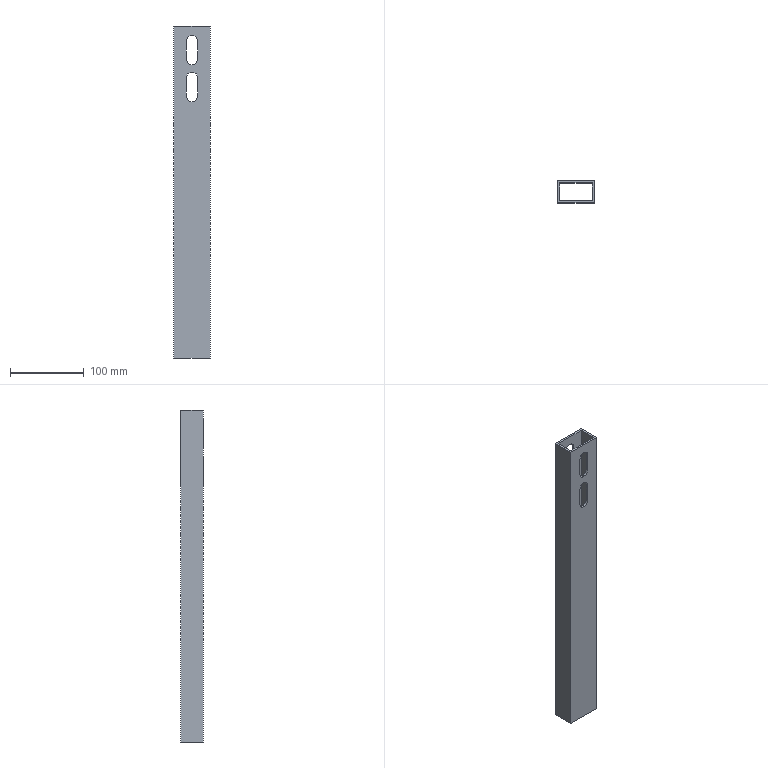Part | SolidWorks | features ICE 2, Extrusion 1 | 1 solid | 30 faces | box 50 x 30 x 450 mm | volume 193179 mm3 | plane 18 | cylinder 12 | commonest cylinder face diameters 15 x12
STEP:
#1=CARTESIAN_POINT('',(32.5,3.,355.));
#2=VERTEX_POINT('',#1);
#3=CARTESIAN_POINT('',(25.,3.,347.5));
#4=VERTEX_POINT('',#3);
#5=CARTESIAN_POINT('',(25.,3.,355.));
#6=DIRECTION('',(0.,1.,0.));
#7=DIRECTION('',(0.,0.,1.));
#8=AXIS2_PLACEMENT_3D('',#5,#6,#7);
#9=CIRCLE('',#8,7.5);
#10=EDGE_CURVE('',#2,#4,#9,.T.);
#11=ORIENTED_EDGE('',*,*,#10,.T.);
#12=CARTESIAN_POINT('',(25.,0.,347.5));
#13=VERTEX_POINT('',#12);
#14=CARTESIAN_POINT('',(25.,450.,347.5));
#15=DIRECTION('',(0.,-1.,0.));
#16=VECTOR('',#15,1000.);
#17=LINE('',#14,#16);
#18=EDGE_CURVE('',#4,#13,#17,.T.);
#19=ORIENTED_EDGE('',*,*,#18,.T.);
#20=CARTESIAN_POINT('',(32.5,0.,355.));
#21=VERTEX_POINT('',#20);
#22=CARTESIAN_POINT('',(25.,0.,355.));
#23=DIRECTION('',(0.,-1.,0.));
#24=DIRECTION('',(0.,0.,-1.));
#25=AXIS2_PLACEMENT_3D('',#22,#23,#24);
#26=CIRCLE('',#25,7.5);
#27=EDGE_CURVE('',#13,#21,#26,.T.);
#28=ORIENTED_EDGE('',*,*,#27,.T.);
#29=CARTESIAN_POINT('',(32.5,450.,355.));
#30=DIRECTION('',(0.,-1.,0.));
#31=VECTOR('',#30,1000.);
#32=LINE('',#29,#31);
#33=EDGE_CURVE('',#2,#21,#32,.T.);
#34=ORIENTED_EDGE('',*,*,#33,.F.);
#35=EDGE_LOOP('',(#11,#19,#28,#34));
#36=FACE_OUTER_BOUND('',#35,.T.);
#37=CARTESIAN_POINT('',(25.,450.,355.));
#38=DIRECTION('',(0.,-1.,0.));
#39=DIRECTION('',(0.,0.,-1.));
#40=AXIS2_PLACEMENT_3D('',#37,#38,#39);
#41=CYLINDRICAL_SURFACE('',#40,7.5);
#42=ADVANCED_FACE('',(#36),#41,.F.);
#43=CARTESIAN_POINT('',(25.,30.,347.5));
#44=VERTEX_POINT('',#43);
#45=CARTESIAN_POINT('',(32.5,30.,355.));
#46=VERTEX_POINT('',#45);
#47=CARTESIAN_POINT('',(25.,30.,355.));
#48=DIRECTION('',(0.,-1.,0.));
#49=DIRECTION('',(0.,0.,-1.));
#50=AXIS2_PLACEMENT_3D('',#47,#48,#49);
#51=CIRCLE('',#50,7.5);
#52=EDGE_CURVE('',#44,#46,#51,.T.);
#53=ORIENTED_EDGE('',*,*,#52,.F.);
#54=CARTESIAN_POINT('',(25.,27.,347.5));
#55=VERTEX_POINT('',#54);
#56=CARTESIAN_POINT('',(25.,450.,347.5));
#57=DIRECTION('',(0.,-1.,0.));
#58=VECTOR('',#57,1000.);
#59=LINE('',#56,#58);
#60=EDGE_CURVE('',#44,#55,#59,.T.);
#61=ORIENTED_EDGE('',*,*,#60,.T.);
#62=CARTESIAN_POINT('',(32.5,27.,355.));
#63=VERTEX_POINT('',#62);
#64=CARTESIAN_POINT('',(25.,27.,355.));
#65=DIRECTION('',(0.,-1.,0.));
#66=DIRECTION('',(0.,0.,-1.));
#67=AXIS2_PLACEMENT_3D('',#64,#65,#66);
#68=CIRCLE('',#67,7.5);
#69=EDGE_CURVE('',#55,#63,#68,.T.);
#70=ORIENTED_EDGE('',*,*,#69,.T.);
#71=CARTESIAN_POINT('',(32.5,450.,355.));
#72=DIRECTION('',(0.,-1.,0.));
#73=VECTOR('',#72,1000.);
#74=LINE('',#71,#73);
#75=EDGE_CURVE('',#46,#63,#74,.T.);
#76=ORIENTED_EDGE('',*,*,#75,.F.);
#77=EDGE_LOOP('',(#53,#61,#70,#76));
#78=FACE_OUTER_BOUND('',#77,.T.);
#79=CARTESIAN_POINT('',(25.,450.,355.));
#80=DIRECTION('',(0.,-1.,0.));
#81=DIRECTION('',(0.,0.,-1.));
#82=AXIS2_PLACEMENT_3D('',#79,#80,#81);
#83=CYLINDRICAL_SURFACE('',#82,7.5);
#84=ADVANCED_FACE('',(#78),#83,.F.);
#85=CARTESIAN_POINT('',(32.5,3.,405.));
#86=VERTEX_POINT('',#85);
#87=CARTESIAN_POINT('',(25.,3.,397.5));
#88=VERTEX_POINT('',#87);
#89=CARTESIAN_POINT('',(25.,3.,405.));
#90=DIRECTION('',(0.,1.,0.));
#91=DIRECTION('',(0.,0.,1.));
#92=AXIS2_PLACEMENT_3D('',#89,#90,#91);
#93=CIRCLE('',#92,7.5);
#94=EDGE_CURVE('',#86,#88,#93,.T.);
#95=ORIENTED_EDGE('',*,*,#94,.T.);
#96=CARTESIAN_POINT('',(25.,0.,397.5));
#97=VERTEX_POINT('',#96);
#98=CARTESIAN_POINT('',(25.,450.,397.5));
#99=DIRECTION('',(0.,-1.,0.));
#100=VECTOR('',#99,1000.);
#101=LINE('',#98,#100);
#102=EDGE_CURVE('',#88,#97,#101,.T.);
#103=ORIENTED_EDGE('',*,*,#102,.T.);
#104=CARTESIAN_POINT('',(32.5,0.,405.));
#105=VERTEX_POINT('',#104);
#106=CARTESIAN_POINT('',(25.,0.,405.));
#107=DIRECTION('',(0.,-1.,0.));
#108=DIRECTION('',(0.,0.,-1.));
#109=AXIS2_PLACEMENT_3D('',#106,#107,#108);
#110=CIRCLE('',#109,7.5);
#111=EDGE_CURVE('',#97,#105,#110,.T.);
#112=ORIENTED_EDGE('',*,*,#111,.T.);
#113=CARTESIAN_POINT('',(32.5,450.,405.));
#114=DIRECTION('',(0.,-1.,0.));
#115=VECTOR('',#114,1000.);
#116=LINE('',#113,#115);
#117=EDGE_CURVE('',#86,#105,#116,.T.);
#118=ORIENTED_EDGE('',*,*,#117,.F.);
#119=EDGE_LOOP('',(#95,#103,#112,#118));
#120=FACE_OUTER_BOUND('',#119,.T.);
#121=CARTESIAN_POINT('',(25.,450.,405.));
#122=DIRECTION('',(0.,-1.,0.));
#123=DIRECTION('',(0.,0.,-1.));
#124=AXIS2_PLACEMENT_3D('',#121,#122,#123);
#125=CYLINDRICAL_SURFACE('',#124,7.5);
#126=ADVANCED_FACE('',(#120),#125,.F.);
#127=CARTESIAN_POINT('',(25.,30.,397.5));
#128=VERTEX_POINT('',#127);
#129=CARTESIAN_POINT('',(32.5,30.,405.));
#130=VERTEX_POINT('',#129);
#131=CARTESIAN_POINT('',(25.,30.,405.));
#132=DIRECTION('',(0.,-1.,0.));
#133=DIRECTION('',(0.,0.,-1.));
#134=AXIS2_PLACEMENT_3D('',#131,#132,#133);
#135=CIRCLE('',#134,7.5);
#136=EDGE_CURVE('',#128,#130,#135,.T.);
#137=ORIENTED_EDGE('',*,*,#136,.F.);
#138=CARTESIAN_POINT('',(25.,27.,397.5));
#139=VERTEX_POINT('',#138);
#140=CARTESIAN_POINT('',(25.,450.,397.5));
#141=DIRECTION('',(0.,-1.,0.));
#142=VECTOR('',#141,1000.);
#143=LINE('',#140,#142);
#144=EDGE_CURVE('',#128,#139,#143,.T.);
#145=ORIENTED_EDGE('',*,*,#144,.T.);
#146=CARTESIAN_POINT('',(32.5,27.,405.));
#147=VERTEX_POINT('',#146);
#148=CARTESIAN_POINT('',(25.,27.,405.));
#149=DIRECTION('',(0.,-1.,0.));
#150=DIRECTION('',(0.,0.,-1.));
#151=AXIS2_PLACEMENT_3D('',#148,#149,#150);
#152=CIRCLE('',#151,7.5);
#153=EDGE_CURVE('',#139,#147,#152,.T.);
#154=ORIENTED_EDGE('',*,*,#153,.T.);
#155=CARTESIAN_POINT('',(32.5,450.,405.));
#156=DIRECTION('',(0.,-1.,0.));
#157=VECTOR('',#156,1000.);
#158=LINE('',#155,#157);
#159=EDGE_CURVE('',#130,#147,#158,.T.);
#160=ORIENTED_EDGE('',*,*,#159,.F.);
#161=EDGE_LOOP('',(#137,#145,#154,#160));
#162=FACE_OUTER_BOUND('',#161,.T.);
#163=CARTESIAN_POINT('',(25.,450.,405.));
#164=DIRECTION('',(0.,-1.,0.));
#165=DIRECTION('',(0.,0.,-1.));
#166=AXIS2_PLACEMENT_3D('',#163,#164,#165);
#167=CYLINDRICAL_SURFACE('',#166,7.5);
#168=ADVANCED_FACE('',(#162),#167,.F.);
#169=CARTESIAN_POINT('',(0.,30.,450.));
#170=VERTEX_POINT('',#169);
#171=CARTESIAN_POINT('',(0.,0.,450.));
#172=VERTEX_POINT('',#171);
#173=CARTESIAN_POINT('',(0.,30.,450.));
#174=DIRECTION('',(0.,-1.,0.));
#175=VECTOR('',#174,1000.);
#176=LINE('',#173,#175);
#177=EDGE_CURVE('',#170,#172,#176,.T.);
#178=ORIENTED_EDGE('',*,*,#177,.T.);
#179=CARTESIAN_POINT('',(50.,0.,450.));
#180=VERTEX_POINT('',#179);
#181=CARTESIAN_POINT('',(0.,0.,450.));
#182=DIRECTION('',(1.,0.,0.));
#183=VECTOR('',#182,1000.);
#184=LINE('',#181,#183);
#185=EDGE_CURVE('',#172,#180,#184,.T.);
#186=ORIENTED_EDGE('',*,*,#185,.T.);
#187=CARTESIAN_POINT('',(50.,30.,450.));
#188=VERTEX_POINT('',#187);
#189=CARTESIAN_POINT('',(50.,0.,450.));
#190=DIRECTION('',(0.,1.,0.));
#191=VECTOR('',#190,1000.);
#192=LINE('',#189,#191);
#193=EDGE_CURVE('',#180,#188,#192,.T.);
#194=ORIENTED_EDGE('',*,*,#193,.T.);
#195=CARTESIAN_POINT('',(50.,30.,450.));
#196=DIRECTION('',(-1.,0.,0.));
#197=VECTOR('',#196,1000.);
#198=LINE('',#195,#197);
#199=EDGE_CURVE('',#188,#170,#198,.T.);
#200=ORIENTED_EDGE('',*,*,#199,.T.);
#201=EDGE_LOOP('',(#178,#186,#194,#200));
#202=FACE_OUTER_BOUND('',#201,.T.);
#203=CARTESIAN_POINT('',(3.,3.,450.));
#204=VERTEX_POINT('',#203);
#205=CARTESIAN_POINT('',(47.,3.,450.));
#206=VERTEX_POINT('',#205);
#207=CARTESIAN_POINT('',(3.,3.,450.));
#208=DIRECTION('',(1.,0.,0.));
#209=VECTOR('',#208,1000.);
#210=LINE('',#207,#209);
#211=EDGE_CURVE('',#204,#206,#210,.T.);
#212=ORIENTED_EDGE('',*,*,#211,.F.);
#213=CARTESIAN_POINT('',(3.,27.,450.));
#214=VERTEX_POINT('',#213);
#215=CARTESIAN_POINT('',(3.,27.,450.));
#216=DIRECTION('',(0.,-1.,0.));
#217=VECTOR('',#216,1000.);
#218=LINE('',#215,#217);
#219=EDGE_CURVE('',#214,#204,#218,.T.);
#220=ORIENTED_EDGE('',*,*,#219,.F.);
#221=CARTESIAN_POINT('',(47.,27.,450.));
#222=VERTEX_POINT('',#221);
#223=CARTESIAN_POINT('',(47.,27.,450.));
#224=DIRECTION('',(-1.,0.,0.));
#225=VECTOR('',#224,1000.);
#226=LINE('',#223,#225);
#227=EDGE_CURVE('',#222,#214,#226,.T.);
#228=ORIENTED_EDGE('',*,*,#227,.F.);
#229=CARTESIAN_POINT('',(47.,3.,450.));
#230=DIRECTION('',(0.,1.,0.));
#231=VECTOR('',#230,1000.);
#232=LINE('',#229,#231);
#233=EDGE_CURVE('',#206,#222,#232,.T.);
#234=ORIENTED_EDGE('',*,*,#233,.F.);
#235=EDGE_LOOP('',(#212,#220,#228,#234));
#236=FACE_BOUND('',#235,.T.);
#237=CARTESIAN_POINT('',(0.,0.,450.));
#238=DIRECTION('',(0.,0.,1.));
#239=DIRECTION('',(1.,0.,0.));
#240=AXIS2_PLACEMENT_3D('',#237,#238,#239);
#241=PLANE('',#240);
#242=ADVANCED_FACE('',(#202,#236),#241,.T.);
#243=CARTESIAN_POINT('',(0.,30.,0.));
#244=VERTEX_POINT('',#243);
#245=CARTESIAN_POINT('',(0.,0.,0.));
#246=VERTEX_POINT('',#245);
#247=CARTESIAN_POINT('',(0.,30.,0.));
#248=DIRECTION('',(0.,-1.,0.));
#249=VECTOR('',#248,1000.);
#250=LINE('',#247,#249);
#251=EDGE_CURVE('',#244,#246,#250,.T.);
#252=ORIENTED_EDGE('',*,*,#251,.F.);
#253=CARTESIAN_POINT('',(50.,30.,0.));
#254=VERTEX_POINT('',#253);
#255=CARTESIAN_POINT('',(50.,30.,0.));
#256=DIRECTION('',(-1.,0.,0.));
#257=VECTOR('',#256,1000.);
#258=LINE('',#255,#257);
#259=EDGE_CURVE('',#254,#244,#258,.T.);
#260=ORIENTED_EDGE('',*,*,#259,.F.);
#261=CARTESIAN_POINT('',(50.,0.,0.));
#262=VERTEX_POINT('',#261);
#263=CARTESIAN_POINT('',(50.,0.,0.));
#264=DIRECTION('',(0.,1.,0.));
#265=VECTOR('',#264,1000.);
#266=LINE('',#263,#265);
#267=EDGE_CURVE('',#262,#254,#266,.T.);
#268=ORIENTED_EDGE('',*,*,#267,.F.);
#269=CARTESIAN_POINT('',(0.,0.,0.));
#270=DIRECTION('',(1.,0.,0.));
#271=VECTOR('',#270,1000.);
#272=LINE('',#269,#271);
#273=EDGE_CURVE('',#246,#262,#272,.T.);
#274=ORIENTED_EDGE('',*,*,#273,.F.);
#275=EDGE_LOOP('',(#252,#260,#268,#274));
#276=FACE_OUTER_BOUND('',#275,.T.);
#277=CARTESIAN_POINT('',(3.,27.,0.));
#278=VERTEX_POINT('',#277);
#279=CARTESIAN_POINT('',(3.,3.,0.));
#280=VERTEX_POINT('',#279);
#281=CARTESIAN_POINT('',(3.,27.,0.));
#282=DIRECTION('',(0.,-1.,0.));
#283=VECTOR('',#282,1000.);
#284=LINE('',#281,#283);
#285=EDGE_CURVE('',#278,#280,#284,.T.);
#286=ORIENTED_EDGE('',*,*,#285,.T.);
#287=CARTESIAN_POINT('',(47.,3.,0.));
#288=VERTEX_POINT('',#287);
#289=CARTESIAN_POINT('',(3.,3.,0.));
#290=DIRECTION('',(1.,0.,0.));
#291=VECTOR('',#290,1000.);
#292=LINE('',#289,#291);
#293=EDGE_CURVE('',#280,#288,#292,.T.);
#294=ORIENTED_EDGE('',*,*,#293,.T.);
#295=CARTESIAN_POINT('',(47.,27.,0.));
#296=VERTEX_POINT('',#295);
#297=CARTESIAN_POINT('',(47.,3.,0.));
#298=DIRECTION('',(0.,1.,0.));
#299=VECTOR('',#298,1000.);
#300=LINE('',#297,#299);
#301=EDGE_CURVE('',#288,#296,#300,.T.);
#302=ORIENTED_EDGE('',*,*,#301,.T.);
#303=CARTESIAN_POINT('',(47.,27.,0.));
#304=DIRECTION('',(-1.,0.,0.));
#305=VECTOR('',#304,1000.);
#306=LINE('',#303,#305);
#307=EDGE_CURVE('',#296,#278,#306,.T.);
#308=ORIENTED_EDGE('',*,*,#307,.T.);
#309=EDGE_LOOP('',(#286,#294,#302,#308));
#310=FACE_BOUND('',#309,.T.);
#311=CARTESIAN_POINT('',(0.,0.,0.));
#312=DIRECTION('',(0.,0.,1.));
#313=DIRECTION('',(1.,0.,0.));
#314=AXIS2_PLACEMENT_3D('',#311,#312,#313);
#315=PLANE('',#314);
#316=ADVANCED_FACE('',(#276,#310),#315,.F.);
#317=ORIENTED_EDGE('',*,*,#251,.T.);
#318=CARTESIAN_POINT('',(0.,0.,450.));
#319=DIRECTION('',(0.,0.,-1.));
#320=VECTOR('',#319,1000.);
#321=LINE('',#318,#320);
#322=EDGE_CURVE('',#172,#246,#321,.T.);
#323=ORIENTED_EDGE('',*,*,#322,.F.);
#324=ORIENTED_EDGE('',*,*,#177,.F.);
#325=CARTESIAN_POINT('',(0.,30.,450.));
#326=DIRECTION('',(0.,0.,-1.));
#327=VECTOR('',#326,1000.);
#328=LINE('',#325,#327);
#329=EDGE_CURVE('',#170,#244,#328,.T.);
#330=ORIENTED_EDGE('',*,*,#329,.T.);
#331=EDGE_LOOP('',(#317,#323,#324,#330));
#332=FACE_OUTER_BOUND('',#331,.T.);
#333=CARTESIAN_POINT('',(0.,30.,450.));
#334=DIRECTION('',(1.,0.,0.));
#335=DIRECTION('',(0.,0.,-1.));
#336=AXIS2_PLACEMENT_3D('',#333,#334,#335);
#337=PLANE('',#336);
#338=ADVANCED_FACE('',(#332),#337,.F.);
#339=CARTESIAN_POINT('',(32.5,0.,380.));
#340=VERTEX_POINT('',#339);
#341=CARTESIAN_POINT('',(32.5,0.,380.));
#342=DIRECTION('',(0.,0.,1.));
#343=VECTOR('',#342,1000.);
#344=LINE('',#341,#343);
#345=EDGE_CURVE('',#21,#340,#344,.T.);
#346=ORIENTED_EDGE('',*,*,#345,.F.);
#347=ORIENTED_EDGE('',*,*,#27,.F.);
#348=CARTESIAN_POINT('',(17.5,0.,355.));
#349=VERTEX_POINT('',#348);
#350=CARTESIAN_POINT('',(25.,0.,355.));
#351=DIRECTION('',(0.,-1.,0.));
#352=DIRECTION('',(0.,0.,-1.));
#353=AXIS2_PLACEMENT_3D('',#350,#351,#352);
#354=CIRCLE('',#353,7.5);
#355=EDGE_CURVE('',#349,#13,#354,.T.);
#356=ORIENTED_EDGE('',*,*,#355,.F.);
#357=CARTESIAN_POINT('',(17.5,0.,380.));
#358=VERTEX_POINT('',#357);
#359=CARTESIAN_POINT('',(17.5,0.,380.));
#360=DIRECTION('',(0.,0.,-1.));
#361=VECTOR('',#360,1000.);
#362=LINE('',#359,#361);
#363=EDGE_CURVE('',#358,#349,#362,.T.);
#364=ORIENTED_EDGE('',*,*,#363,.F.);
#365=CARTESIAN_POINT('',(25.,0.,380.));
#366=DIRECTION('',(0.,-1.,0.));
#367=DIRECTION('',(0.,0.,-1.));
#368=AXIS2_PLACEMENT_3D('',#365,#366,#367);
#369=CIRCLE('',#368,7.5);
#370=EDGE_CURVE('',#340,#358,#369,.T.);
#371=ORIENTED_EDGE('',*,*,#370,.F.);
#372=EDGE_LOOP('',(#346,#347,#356,#364,#371));
#373=FACE_BOUND('',#372,.T.);
#374=CARTESIAN_POINT('',(17.5,0.,430.));
#375=VERTEX_POINT('',#374);
#376=CARTESIAN_POINT('',(17.5,0.,405.));
#377=VERTEX_POINT('',#376);
#378=CARTESIAN_POINT('',(17.5,0.,430.));
#379=DIRECTION('',(0.,0.,-1.));
#380=VECTOR('',#379,1000.);
#381=LINE('',#378,#380);
#382=EDGE_CURVE('',#375,#377,#381,.T.);
#383=ORIENTED_EDGE('',*,*,#382,.F.);
#384=CARTESIAN_POINT('',(32.5,0.,430.));
#385=VERTEX_POINT('',#384);
#386=CARTESIAN_POINT('',(25.,0.,430.));
#387=DIRECTION('',(0.,-1.,0.));
#388=DIRECTION('',(0.,0.,-1.));
#389=AXIS2_PLACEMENT_3D('',#386,#387,#388);
#390=CIRCLE('',#389,7.5);
#391=EDGE_CURVE('',#385,#375,#390,.T.);
#392=ORIENTED_EDGE('',*,*,#391,.F.);
#393=CARTESIAN_POINT('',(32.5,0.,430.));
#394=DIRECTION('',(0.,0.,1.));
#395=VECTOR('',#394,1000.);
#396=LINE('',#393,#395);
#397=EDGE_CURVE('',#105,#385,#396,.T.);
#398=ORIENTED_EDGE('',*,*,#397,.F.);
#399=ORIENTED_EDGE('',*,*,#111,.F.);
#400=CARTESIAN_POINT('',(25.,0.,405.));
#401=DIRECTION('',(0.,-1.,0.));
#402=DIRECTION('',(0.,0.,-1.));
#403=AXIS2_PLACEMENT_3D('',#400,#401,#402);
#404=CIRCLE('',#403,7.5);
#405=EDGE_CURVE('',#377,#97,#404,.T.);
#406=ORIENTED_EDGE('',*,*,#405,.F.);
#407=EDGE_LOOP('',(#383,#392,#398,#399,#406));
#408=FACE_BOUND('',#407,.T.);
#409=ORIENTED_EDGE('',*,*,#273,.T.);
#410=CARTESIAN_POINT('',(50.,0.,450.));
#411=DIRECTION('',(0.,0.,-1.));
#412=VECTOR('',#411,1000.);
#413=LINE('',#410,#412);
#414=EDGE_CURVE('',#180,#262,#413,.T.);
#415=ORIENTED_EDGE('',*,*,#414,.F.);
#416=ORIENTED_EDGE('',*,*,#185,.F.);
#417=ORIENTED_EDGE('',*,*,#322,.T.);
#418=EDGE_LOOP('',(#409,#415,#416,#417));
#419=FACE_OUTER_BOUND('',#418,.T.);
#420=CARTESIAN_POINT('',(0.,0.,450.));
#421=DIRECTION('',(0.,1.,0.));
#422=DIRECTION('',(0.,0.,1.));
#423=AXIS2_PLACEMENT_3D('',#420,#421,#422);
#424=PLANE('',#423);
#425=ADVANCED_FACE('',(#373,#408,#419),#424,.F.);
#426=ORIENTED_EDGE('',*,*,#267,.T.);
#427=CARTESIAN_POINT('',(50.,30.,450.));
#428=DIRECTION('',(0.,0.,-1.));
#429=VECTOR('',#428,1000.);
#430=LINE('',#427,#429);
#431=EDGE_CURVE('',#188,#254,#430,.T.);
#432=ORIENTED_EDGE('',*,*,#431,.F.);
#433=ORIENTED_EDGE('',*,*,#193,.F.);
#434=ORIENTED_EDGE('',*,*,#414,.T.);
#435=EDGE_LOOP('',(#426,#432,#433,#434));
#436=FACE_OUTER_BOUND('',#435,.T.);
#437=CARTESIAN_POINT('',(50.,0.,450.));
#438=DIRECTION('',(-1.,0.,0.));
#439=DIRECTION('',(0.,0.,1.));
#440=AXIS2_PLACEMENT_3D('',#437,#438,#439);
#441=PLANE('',#440);
#442=ADVANCED_FACE('',(#436),#441,.F.);
#443=CARTESIAN_POINT('',(17.5,30.,380.));
#444=VERTEX_POINT('',#443);
#445=CARTESIAN_POINT('',(17.5,30.,355.));
#446=VERTEX_POINT('',#445);
#447=CARTESIAN_POINT('',(17.5,30.,450.));
#448=DIRECTION('',(0.,0.,-1.));
#449=VECTOR('',#448,1000.);
#450=LINE('',#447,#449);
#451=EDGE_CURVE('',#444,#446,#450,.T.);
#452=ORIENTED_EDGE('',*,*,#451,.T.);
#453=CARTESIAN_POINT('',(25.,30.,355.));
#454=DIRECTION('',(0.,-1.,0.));
#455=DIRECTION('',(0.,0.,-1.));
#456=AXIS2_PLACEMENT_3D('',#453,#454,#455);
#457=CIRCLE('',#456,7.5);
#458=EDGE_CURVE('',#446,#44,#457,.T.);
#459=ORIENTED_EDGE('',*,*,#458,.T.);
#460=ORIENTED_EDGE('',*,*,#52,.T.);
#461=CARTESIAN_POINT('',(32.5,30.,380.));
#462=VERTEX_POINT('',#461);
#463=CARTESIAN_POINT('',(32.5,30.,450.));
#464=DIRECTION('',(0.,0.,1.));
#465=VECTOR('',#464,1000.);
#466=LINE('',#463,#465);
#467=EDGE_CURVE('',#46,#462,#466,.T.);
#468=ORIENTED_EDGE('',*,*,#467,.T.);
#469=CARTESIAN_POINT('',(25.,30.,380.));
#470=DIRECTION('',(0.,-1.,0.));
#471=DIRECTION('',(0.,0.,-1.));
#472=AXIS2_PLACEMENT_3D('',#469,#470,#471);
#473=CIRCLE('',#472,7.5);
#474=EDGE_CURVE('',#462,#444,#473,.T.);
#475=ORIENTED_EDGE('',*,*,#474,.T.);
#476=EDGE_LOOP('',(#452,#459,#460,#468,#475));
#477=FACE_BOUND('',#476,.T.);
#478=CARTESIAN_POINT('',(32.5,30.,430.));
#479=VERTEX_POINT('',#478);
#480=CARTESIAN_POINT('',(32.5,30.,450.));
#481=DIRECTION('',(0.,0.,1.));
#482=VECTOR('',#481,1000.);
#483=LINE('',#480,#482);
#484=EDGE_CURVE('',#130,#479,#483,.T.);
#485=ORIENTED_EDGE('',*,*,#484,.T.);
#486=CARTESIAN_POINT('',(17.5,30.,430.));
#487=VERTEX_POINT('',#486);
#488=CARTESIAN_POINT('',(25.,30.,430.));
#489=DIRECTION('',(0.,-1.,0.));
#490=DIRECTION('',(0.,0.,-1.));
#491=AXIS2_PLACEMENT_3D('',#488,#489,#490);
#492=CIRCLE('',#491,7.5);
#493=EDGE_CURVE('',#479,#487,#492,.T.);
#494=ORIENTED_EDGE('',*,*,#493,.T.);
#495=CARTESIAN_POINT('',(17.5,30.,405.));
#496=VERTEX_POINT('',#495);
#497=CARTESIAN_POINT('',(17.5,30.,450.));
#498=DIRECTION('',(0.,0.,-1.));
#499=VECTOR('',#498,1000.);
#500=LINE('',#497,#499);
#501=EDGE_CURVE('',#487,#496,#500,.T.);
#502=ORIENTED_EDGE('',*,*,#501,.T.);
#503=CARTESIAN_POINT('',(25.,30.,405.));
#504=DIRECTION('',(0.,-1.,0.));
#505=DIRECTION('',(0.,0.,-1.));
#506=AXIS2_PLACEMENT_3D('',#503,#504,#505);
#507=CIRCLE('',#506,7.5);
#508=EDGE_CURVE('',#496,#128,#507,.T.);
#509=ORIENTED_EDGE('',*,*,#508,.T.);
#510=ORIENTED_EDGE('',*,*,#136,.T.);
#511=EDGE_LOOP('',(#485,#494,#502,#509,#510));
#512=FACE_BOUND('',#511,.T.);
#513=ORIENTED_EDGE('',*,*,#259,.T.);
#514=ORIENTED_EDGE('',*,*,#329,.F.);
#515=ORIENTED_EDGE('',*,*,#199,.F.);
#516=ORIENTED_EDGE('',*,*,#431,.T.);
#517=EDGE_LOOP('',(#513,#514,#515,#516));
#518=FACE_OUTER_BOUND('',#517,.T.);
#519=CARTESIAN_POINT('',(50.,30.,450.));
#520=DIRECTION('',(0.,-1.,0.));
#521=DIRECTION('',(0.,0.,-1.));
#522=AXIS2_PLACEMENT_3D('',#519,#520,#521);
#523=PLANE('',#522);
#524=ADVANCED_FACE('',(#477,#512,#518),#523,.F.);
#525=ORIENTED_EDGE('',*,*,#285,.F.);
#526=CARTESIAN_POINT('',(3.,27.,450.));
#527=DIRECTION('',(0.,0.,-1.));
#528=VECTOR('',#527,1000.);
#529=LINE('',#526,#528);
#530=EDGE_CURVE('',#214,#278,#529,.T.);
#531=ORIENTED_EDGE('',*,*,#530,.F.);
#532=ORIENTED_EDGE('',*,*,#219,.T.);
#533=CARTESIAN_POINT('',(3.,3.,450.));
#534=DIRECTION('',(0.,0.,-1.));
#535=VECTOR('',#534,1000.);
#536=LINE('',#533,#535);
#537=EDGE_CURVE('',#204,#280,#536,.T.);
#538=ORIENTED_EDGE('',*,*,#537,.T.);
#539=EDGE_LOOP('',(#525,#531,#532,#538));
#540=FACE_OUTER_BOUND('',#539,.T.);
#541=CARTESIAN_POINT('',(3.,27.,450.));
#542=DIRECTION('',(1.,0.,0.));
#543=DIRECTION('',(0.,0.,-1.));
#544=AXIS2_PLACEMENT_3D('',#541,#542,#543);
#545=PLANE('',#544);
#546=ADVANCED_FACE('',(#540),#545,.T.);
#547=ORIENTED_EDGE('',*,*,#10,.F.);
#548=CARTESIAN_POINT('',(32.5,3.,380.));
#549=VERTEX_POINT('',#548);
#550=CARTESIAN_POINT('',(32.5,3.,450.));
#551=DIRECTION('',(0.,0.,-1.));
#552=VECTOR('',#551,1000.);
#553=LINE('',#550,#552);
#554=EDGE_CURVE('',#549,#2,#553,.T.);
#555=ORIENTED_EDGE('',*,*,#554,.F.);
#556=CARTESIAN_POINT('',(17.5,3.,380.));
#557=VERTEX_POINT('',#556);
#558=CARTESIAN_POINT('',(25.,3.,380.));
#559=DIRECTION('',(0.,1.,0.));
#560=DIRECTION('',(0.,0.,1.));
#561=AXIS2_PLACEMENT_3D('',#558,#559,#560);
#562=CIRCLE('',#561,7.5);
#563=EDGE_CURVE('',#557,#549,#562,.T.);
#564=ORIENTED_EDGE('',*,*,#563,.F.);
#565=CARTESIAN_POINT('',(17.5,3.,355.));
#566=VERTEX_POINT('',#565);
#567=CARTESIAN_POINT('',(17.5,3.,450.));
#568=DIRECTION('',(0.,0.,1.));
#569=VECTOR('',#568,1000.);
#570=LINE('',#567,#569);
#571=EDGE_CURVE('',#566,#557,#570,.T.);
#572=ORIENTED_EDGE('',*,*,#571,.F.);
#573=CARTESIAN_POINT('',(25.,3.,355.));
#574=DIRECTION('',(0.,1.,0.));
#575=DIRECTION('',(0.,0.,1.));
#576=AXIS2_PLACEMENT_3D('',#573,#574,#575);
#577=CIRCLE('',#576,7.5);
#578=EDGE_CURVE('',#4,#566,#577,.T.);
#579=ORIENTED_EDGE('',*,*,#578,.F.);
#580=EDGE_LOOP('',(#547,#555,#564,#572,#579));
#581=FACE_BOUND('',#580,.T.);
#582=CARTESIAN_POINT('',(17.5,3.,430.));
#583=VERTEX_POINT('',#582);
#584=CARTESIAN_POINT('',(32.5,3.,430.));
#585=VERTEX_POINT('',#584);
#586=CARTESIAN_POINT('',(25.,3.,430.));
#587=DIRECTION('',(0.,1.,0.));
#588=DIRECTION('',(0.,0.,1.));
#589=AXIS2_PLACEMENT_3D('',#586,#587,#588);
#590=CIRCLE('',#589,7.5);
#591=EDGE_CURVE('',#583,#585,#590,.T.);
#592=ORIENTED_EDGE('',*,*,#591,.F.);
#593=CARTESIAN_POINT('',(17.5,3.,405.));
#594=VERTEX_POINT('',#593);
#595=CARTESIAN_POINT('',(17.5,3.,450.));
#596=DIRECTION('',(0.,0.,1.));
#597=VECTOR('',#596,1000.);
#598=LINE('',#595,#597);
#599=EDGE_CURVE('',#594,#583,#598,.T.);
#600=ORIENTED_EDGE('',*,*,#599,.F.);
#601=CARTESIAN_POINT('',(25.,3.,405.));
#602=DIRECTION('',(0.,1.,0.));
#603=DIRECTION('',(0.,0.,1.));
#604=AXIS2_PLACEMENT_3D('',#601,#602,#603);
#605=CIRCLE('',#604,7.5);
#606=EDGE_CURVE('',#88,#594,#605,.T.);
#607=ORIENTED_EDGE('',*,*,#606,.F.);
#608=ORIENTED_EDGE('',*,*,#94,.F.);
#609=CARTESIAN_POINT('',(32.5,3.,450.));
#610=DIRECTION('',(0.,0.,-1.));
#611=VECTOR('',#610,1000.);
#612=LINE('',#609,#611);
#613=EDGE_CURVE('',#585,#86,#612,.T.);
#614=ORIENTED_EDGE('',*,*,#613,.F.);
#615=EDGE_LOOP('',(#592,#600,#607,#608,#614));
#616=FACE_BOUND('',#615,.T.);
#617=ORIENTED_EDGE('',*,*,#293,.F.);
#618=ORIENTED_EDGE('',*,*,#537,.F.);
#619=ORIENTED_EDGE('',*,*,#211,.T.);
#620=CARTESIAN_POINT('',(47.,3.,450.));
#621=DIRECTION('',(0.,0.,-1.));
#622=VECTOR('',#621,1000.);
#623=LINE('',#620,#622);
#624=EDGE_CURVE('',#206,#288,#623,.T.);
#625=ORIENTED_EDGE('',*,*,#624,.T.);
#626=EDGE_LOOP('',(#617,#618,#619,#625));
#627=FACE_OUTER_BOUND('',#626,.T.);
#628=CARTESIAN_POINT('',(3.,3.,450.));
#629=DIRECTION('',(0.,1.,0.));
#630=DIRECTION('',(0.,0.,1.));
#631=AXIS2_PLACEMENT_3D('',#628,#629,#630);
#632=PLANE('',#631);
#633=ADVANCED_FACE('',(#581,#616,#627),#632,.T.);
#634=ORIENTED_EDGE('',*,*,#301,.F.);
#635=ORIENTED_EDGE('',*,*,#624,.F.);
#636=ORIENTED_EDGE('',*,*,#233,.T.);
#637=CARTESIAN_POINT('',(47.,27.,450.));
#638=DIRECTION('',(0.,0.,-1.));
#639=VECTOR('',#638,1000.);
#640=LINE('',#637,#639);
#641=EDGE_CURVE('',#222,#296,#640,.T.);
#642=ORIENTED_EDGE('',*,*,#641,.T.);
#643=EDGE_LOOP('',(#634,#635,#636,#642));
#644=FACE_OUTER_BOUND('',#643,.T.);
#645=CARTESIAN_POINT('',(47.,3.,450.));
#646=DIRECTION('',(-1.,0.,0.));
#647=DIRECTION('',(0.,0.,1.));
#648=AXIS2_PLACEMENT_3D('',#645,#646,#647);
#649=PLANE('',#648);
#650=ADVANCED_FACE('',(#644),#649,.T.);
#651=CARTESIAN_POINT('',(17.5,27.,355.));
#652=VERTEX_POINT('',#651);
#653=CARTESIAN_POINT('',(25.,27.,355.));
#654=DIRECTION('',(0.,-1.,0.));
#655=DIRECTION('',(0.,0.,-1.));
#656=AXIS2_PLACEMENT_3D('',#653,#654,#655);
#657=CIRCLE('',#656,7.5);
#658=EDGE_CURVE('',#652,#55,#657,.T.);
#659=ORIENTED_EDGE('',*,*,#658,.F.);
#660=CARTESIAN_POINT('',(17.5,27.,380.));
#661=VERTEX_POINT('',#660);
#662=CARTESIAN_POINT('',(17.5,27.,450.));
#663=DIRECTION('',(0.,0.,-1.));
#664=VECTOR('',#663,1000.);
#665=LINE('',#662,#664);
#666=EDGE_CURVE('',#661,#652,#665,.T.);
#667=ORIENTED_EDGE('',*,*,#666,.F.);
#668=CARTESIAN_POINT('',(32.5,27.,380.));
#669=VERTEX_POINT('',#668);
#670=CARTESIAN_POINT('',(25.,27.,380.));
#671=DIRECTION('',(0.,-1.,0.));
#672=DIRECTION('',(0.,0.,-1.));
#673=AXIS2_PLACEMENT_3D('',#670,#671,#672);
#674=CIRCLE('',#673,7.5);
#675=EDGE_CURVE('',#669,#661,#674,.T.);
#676=ORIENTED_EDGE('',*,*,#675,.F.);
#677=CARTESIAN_POINT('',(32.5,27.,450.));
#678=DIRECTION('',(0.,0.,1.));
#679=VECTOR('',#678,1000.);
#680=LINE('',#677,#679);
#681=EDGE_CURVE('',#63,#669,#680,.T.);
#682=ORIENTED_EDGE('',*,*,#681,.F.);
#683=ORIENTED_EDGE('',*,*,#69,.F.);
#684=EDGE_LOOP('',(#659,#667,#676,#682,#683));
#685=FACE_BOUND('',#684,.T.);
#686=CARTESIAN_POINT('',(32.5,27.,430.));
#687=VERTEX_POINT('',#686);
#688=CARTESIAN_POINT('',(17.5,27.,430.));
#689=VERTEX_POINT('',#688);
#690=CARTESIAN_POINT('',(25.,27.,430.));
#691=DIRECTION('',(0.,-1.,0.));
#692=DIRECTION('',(0.,0.,-1.));
#693=AXIS2_PLACEMENT_3D('',#690,#691,#692);
#694=CIRCLE('',#693,7.5);
#695=EDGE_CURVE('',#687,#689,#694,.T.);
#696=ORIENTED_EDGE('',*,*,#695,.F.);
#697=CARTESIAN_POINT('',(32.5,27.,450.));
#698=DIRECTION('',(0.,0.,1.));
#699=VECTOR('',#698,1000.);
#700=LINE('',#697,#699);
#701=EDGE_CURVE('',#147,#687,#700,.T.);
#702=ORIENTED_EDGE('',*,*,#701,.F.);
#703=ORIENTED_EDGE('',*,*,#153,.F.);
#704=CARTESIAN_POINT('',(17.5,27.,405.));
#705=VERTEX_POINT('',#704);
#706=CARTESIAN_POINT('',(25.,27.,405.));
#707=DIRECTION('',(0.,-1.,0.));
#708=DIRECTION('',(0.,0.,-1.));
#709=AXIS2_PLACEMENT_3D('',#706,#707,#708);
#710=CIRCLE('',#709,7.5);
#711=EDGE_CURVE('',#705,#139,#710,.T.);
#712=ORIENTED_EDGE('',*,*,#711,.F.);
#713=CARTESIAN_POINT('',(17.5,27.,450.));
#714=DIRECTION('',(0.,0.,-1.));
#715=VECTOR('',#714,1000.);
#716=LINE('',#713,#715);
#717=EDGE_CURVE('',#689,#705,#716,.T.);
#718=ORIENTED_EDGE('',*,*,#717,.F.);
#719=EDGE_LOOP('',(#696,#702,#703,#712,#718));
#720=FACE_BOUND('',#719,.T.);
#721=ORIENTED_EDGE('',*,*,#307,.F.);
#722=ORIENTED_EDGE('',*,*,#641,.F.);
#723=ORIENTED_EDGE('',*,*,#227,.T.);
#724=ORIENTED_EDGE('',*,*,#530,.T.);
#725=EDGE_LOOP('',(#721,#722,#723,#724));
#726=FACE_OUTER_BOUND('',#725,.T.);
#727=CARTESIAN_POINT('',(47.,27.,450.));
#728=DIRECTION('',(0.,-1.,0.));
#729=DIRECTION('',(0.,0.,-1.));
#730=AXIS2_PLACEMENT_3D('',#727,#728,#729);
#731=PLANE('',#730);
#732=ADVANCED_FACE('',(#685,#720,#726),#731,.T.);
#733=CARTESIAN_POINT('',(17.5,450.,430.));
#734=DIRECTION('',(0.,-1.,0.));
#735=VECTOR('',#734,1000.);
#736=LINE('',#733,#735);
#737=EDGE_CURVE('',#487,#689,#736,.T.);
#738=ORIENTED_EDGE('',*,*,#737,.T.);
#739=ORIENTED_EDGE('',*,*,#717,.T.);
#740=CARTESIAN_POINT('',(17.5,450.,405.));
#741=DIRECTION('',(0.,-1.,0.));
#742=VECTOR('',#741,1000.);
#743=LINE('',#740,#742);
#744=EDGE_CURVE('',#496,#705,#743,.T.);
#745=ORIENTED_EDGE('',*,*,#744,.F.);
#746=ORIENTED_EDGE('',*,*,#501,.F.);
#747=EDGE_LOOP('',(#738,#739,#745,#746));
#748=FACE_OUTER_BOUND('',#747,.T.);
#749=CARTESIAN_POINT('',(17.5,450.,430.));
#750=DIRECTION('',(-1.,0.,0.));
#751=DIRECTION('',(0.,0.,1.));
#752=AXIS2_PLACEMENT_3D('',#749,#750,#751);
#753=PLANE('',#752);
#754=ADVANCED_FACE('',(#748),#753,.F.);
#755=ORIENTED_EDGE('',*,*,#144,.F.);
#756=ORIENTED_EDGE('',*,*,#508,.F.);
#757=ORIENTED_EDGE('',*,*,#744,.T.);
#758=ORIENTED_EDGE('',*,*,#711,.T.);
#759=EDGE_LOOP('',(#755,#756,#757,#758));
#760=FACE_OUTER_BOUND('',#759,.T.);
#761=CARTESIAN_POINT('',(25.,450.,405.));
#762=DIRECTION('',(0.,-1.,0.));
#763=DIRECTION('',(0.,0.,-1.));
#764=AXIS2_PLACEMENT_3D('',#761,#762,#763);
#765=CYLINDRICAL_SURFACE('',#764,7.5);
#766=ADVANCED_FACE('',(#760),#765,.F.);
#767=ORIENTED_EDGE('',*,*,#159,.T.);
#768=ORIENTED_EDGE('',*,*,#701,.T.);
#769=CARTESIAN_POINT('',(32.5,450.,430.));
#770=DIRECTION('',(0.,-1.,0.));
#771=VECTOR('',#770,1000.);
#772=LINE('',#769,#771);
#773=EDGE_CURVE('',#479,#687,#772,.T.);
#774=ORIENTED_EDGE('',*,*,#773,.F.);
#775=ORIENTED_EDGE('',*,*,#484,.F.);
#776=EDGE_LOOP('',(#767,#768,#774,#775));
#777=FACE_OUTER_BOUND('',#776,.T.);
#778=CARTESIAN_POINT('',(32.5,450.,430.));
#779=DIRECTION('',(1.,0.,0.));
#780=DIRECTION('',(0.,0.,-1.));
#781=AXIS2_PLACEMENT_3D('',#778,#779,#780);
#782=PLANE('',#781);
#783=ADVANCED_FACE('',(#777),#782,.F.);
#784=ORIENTED_EDGE('',*,*,#773,.T.);
#785=ORIENTED_EDGE('',*,*,#695,.T.);
#786=ORIENTED_EDGE('',*,*,#737,.F.);
#787=ORIENTED_EDGE('',*,*,#493,.F.);
#788=EDGE_LOOP('',(#784,#785,#786,#787));
#789=FACE_OUTER_BOUND('',#788,.T.);
#790=CARTESIAN_POINT('',(25.,450.,430.));
#791=DIRECTION('',(0.,-1.,0.));
#792=DIRECTION('',(0.,0.,-1.));
#793=AXIS2_PLACEMENT_3D('',#790,#791,#792);
#794=CYLINDRICAL_SURFACE('',#793,7.5);
#795=ADVANCED_FACE('',(#789),#794,.F.);
#796=ORIENTED_EDGE('',*,*,#591,.T.);
#797=CARTESIAN_POINT('',(32.5,450.,430.));
#798=DIRECTION('',(0.,-1.,0.));
#799=VECTOR('',#798,1000.);
#800=LINE('',#797,#799);
#801=EDGE_CURVE('',#585,#385,#800,.T.);
#802=ORIENTED_EDGE('',*,*,#801,.T.);
#803=ORIENTED_EDGE('',*,*,#391,.T.);
#804=CARTESIAN_POINT('',(17.5,450.,430.));
#805=DIRECTION('',(0.,-1.,0.));
#806=VECTOR('',#805,1000.);
#807=LINE('',#804,#806);
#808=EDGE_CURVE('',#583,#375,#807,.T.);
#809=ORIENTED_EDGE('',*,*,#808,.F.);
#810=EDGE_LOOP('',(#796,#802,#803,#809));
#811=FACE_OUTER_BOUND('',#810,.T.);
#812=CARTESIAN_POINT('',(25.,450.,430.));
#813=DIRECTION('',(0.,-1.,0.));
#814=DIRECTION('',(0.,0.,-1.));
#815=AXIS2_PLACEMENT_3D('',#812,#813,#814);
#816=CYLINDRICAL_SURFACE('',#815,7.5);
#817=ADVANCED_FACE('',(#811),#816,.F.);
#818=ORIENTED_EDGE('',*,*,#613,.T.);
#819=ORIENTED_EDGE('',*,*,#117,.T.);
#820=ORIENTED_EDGE('',*,*,#397,.T.);
#821=ORIENTED_EDGE('',*,*,#801,.F.);
#822=EDGE_LOOP('',(#818,#819,#820,#821));
#823=FACE_OUTER_BOUND('',#822,.T.);
#824=CARTESIAN_POINT('',(32.5,450.,430.));
#825=DIRECTION('',(1.,0.,0.));
#826=DIRECTION('',(0.,0.,-1.));
#827=AXIS2_PLACEMENT_3D('',#824,#825,#826);
#828=PLANE('',#827);
#829=ADVANCED_FACE('',(#823),#828,.F.);
#830=ORIENTED_EDGE('',*,*,#102,.F.);
#831=ORIENTED_EDGE('',*,*,#606,.T.);
#832=CARTESIAN_POINT('',(17.5,450.,405.));
#833=DIRECTION('',(0.,-1.,0.));
#834=VECTOR('',#833,1000.);
#835=LINE('',#832,#834);
#836=EDGE_CURVE('',#594,#377,#835,.T.);
#837=ORIENTED_EDGE('',*,*,#836,.T.);
#838=ORIENTED_EDGE('',*,*,#405,.T.);
#839=EDGE_LOOP('',(#830,#831,#837,#838));
#840=FACE_OUTER_BOUND('',#839,.T.);
#841=CARTESIAN_POINT('',(25.,450.,405.));
#842=DIRECTION('',(0.,-1.,0.));
#843=DIRECTION('',(0.,0.,-1.));
#844=AXIS2_PLACEMENT_3D('',#841,#842,#843);
#845=CYLINDRICAL_SURFACE('',#844,7.5);
#846=ADVANCED_FACE('',(#840),#845,.F.);
#847=ORIENTED_EDGE('',*,*,#599,.T.);
#848=ORIENTED_EDGE('',*,*,#808,.T.);
#849=ORIENTED_EDGE('',*,*,#382,.T.);
#850=ORIENTED_EDGE('',*,*,#836,.F.);
#851=EDGE_LOOP('',(#847,#848,#849,#850));
#852=FACE_OUTER_BOUND('',#851,.T.);
#853=CARTESIAN_POINT('',(17.5,450.,430.));
#854=DIRECTION('',(-1.,0.,0.));
#855=DIRECTION('',(0.,0.,1.));
#856=AXIS2_PLACEMENT_3D('',#853,#854,#855);
#857=PLANE('',#856);
#858=ADVANCED_FACE('',(#852),#857,.F.);
#859=ORIENTED_EDGE('',*,*,#75,.T.);
#860=ORIENTED_EDGE('',*,*,#681,.T.);
#861=CARTESIAN_POINT('',(32.5,450.,380.));
#862=DIRECTION('',(0.,-1.,0.));
#863=VECTOR('',#862,1000.);
#864=LINE('',#861,#863);
#865=EDGE_CURVE('',#462,#669,#864,.T.);
#866=ORIENTED_EDGE('',*,*,#865,.F.);
#867=ORIENTED_EDGE('',*,*,#467,.F.);
#868=EDGE_LOOP('',(#859,#860,#866,#867));
#869=FACE_OUTER_BOUND('',#868,.T.);
#870=CARTESIAN_POINT('',(32.5,450.,380.));
#871=DIRECTION('',(1.,0.,0.));
#872=DIRECTION('',(0.,0.,-1.));
#873=AXIS2_PLACEMENT_3D('',#870,#871,#872);
#874=PLANE('',#873);
#875=ADVANCED_FACE('',(#869),#874,.F.);
#876=ORIENTED_EDGE('',*,*,#865,.T.);
#877=ORIENTED_EDGE('',*,*,#675,.T.);
#878=CARTESIAN_POINT('',(17.5,450.,380.));
#879=DIRECTION('',(0.,-1.,0.));
#880=VECTOR('',#879,1000.);
#881=LINE('',#878,#880);
#882=EDGE_CURVE('',#444,#661,#881,.T.);
#883=ORIENTED_EDGE('',*,*,#882,.F.);
#884=ORIENTED_EDGE('',*,*,#474,.F.);
#885=EDGE_LOOP('',(#876,#877,#883,#884));
#886=FACE_OUTER_BOUND('',#885,.T.);
#887=CARTESIAN_POINT('',(25.,450.,380.));
#888=DIRECTION('',(0.,-1.,0.));
#889=DIRECTION('',(0.,0.,-1.));
#890=AXIS2_PLACEMENT_3D('',#887,#888,#889);
#891=CYLINDRICAL_SURFACE('',#890,7.5);
#892=ADVANCED_FACE('',(#886),#891,.F.);
#893=ORIENTED_EDGE('',*,*,#882,.T.);
#894=ORIENTED_EDGE('',*,*,#666,.T.);
#895=CARTESIAN_POINT('',(17.5,450.,355.));
#896=DIRECTION('',(0.,-1.,0.));
#897=VECTOR('',#896,1000.);
#898=LINE('',#895,#897);
#899=EDGE_CURVE('',#446,#652,#898,.T.);
#900=ORIENTED_EDGE('',*,*,#899,.F.);
#901=ORIENTED_EDGE('',*,*,#451,.F.);
#902=EDGE_LOOP('',(#893,#894,#900,#901));
#903=FACE_OUTER_BOUND('',#902,.T.);
#904=CARTESIAN_POINT('',(17.5,450.,380.));
#905=DIRECTION('',(-1.,0.,0.));
#906=DIRECTION('',(0.,0.,1.));
#907=AXIS2_PLACEMENT_3D('',#904,#905,#906);
#908=PLANE('',#907);
#909=ADVANCED_FACE('',(#903),#908,.F.);
#910=ORIENTED_EDGE('',*,*,#60,.F.);
#911=ORIENTED_EDGE('',*,*,#458,.F.);
#912=ORIENTED_EDGE('',*,*,#899,.T.);
#913=ORIENTED_EDGE('',*,*,#658,.T.);
#914=EDGE_LOOP('',(#910,#911,#912,#913));
#915=FACE_OUTER_BOUND('',#914,.T.);
#916=CARTESIAN_POINT('',(25.,450.,355.));
#917=DIRECTION('',(0.,-1.,0.));
#918=DIRECTION('',(0.,0.,-1.));
#919=AXIS2_PLACEMENT_3D('',#916,#917,#918);
#920=CYLINDRICAL_SURFACE('',#919,7.5);
#921=ADVANCED_FACE('',(#915),#920,.F.);
#922=ORIENTED_EDGE('',*,*,#18,.F.);
#923=ORIENTED_EDGE('',*,*,#578,.T.);
#924=CARTESIAN_POINT('',(17.5,450.,355.));
#925=DIRECTION('',(0.,-1.,0.));
#926=VECTOR('',#925,1000.);
#927=LINE('',#924,#926);
#928=EDGE_CURVE('',#566,#349,#927,.T.);
#929=ORIENTED_EDGE('',*,*,#928,.T.);
#930=ORIENTED_EDGE('',*,*,#355,.T.);
#931=EDGE_LOOP('',(#922,#923,#929,#930));
#932=FACE_OUTER_BOUND('',#931,.T.);
#933=CARTESIAN_POINT('',(25.,450.,355.));
#934=DIRECTION('',(0.,-1.,0.));
#935=DIRECTION('',(0.,0.,-1.));
#936=AXIS2_PLACEMENT_3D('',#933,#934,#935);
#937=CYLINDRICAL_SURFACE('',#936,7.5);
#938=ADVANCED_FACE('',(#932),#937,.F.);
#939=ORIENTED_EDGE('',*,*,#571,.T.);
#940=CARTESIAN_POINT('',(17.5,450.,380.));
#941=DIRECTION('',(0.,-1.,0.));
#942=VECTOR('',#941,1000.);
#943=LINE('',#940,#942);
#944=EDGE_CURVE('',#557,#358,#943,.T.);
#945=ORIENTED_EDGE('',*,*,#944,.T.);
#946=ORIENTED_EDGE('',*,*,#363,.T.);
#947=ORIENTED_EDGE('',*,*,#928,.F.);
#948=EDGE_LOOP('',(#939,#945,#946,#947));
#949=FACE_OUTER_BOUND('',#948,.T.);
#950=CARTESIAN_POINT('',(17.5,450.,380.));
#951=DIRECTION('',(-1.,0.,0.));
#952=DIRECTION('',(0.,0.,1.));
#953=AXIS2_PLACEMENT_3D('',#950,#951,#952);
#954=PLANE('',#953);
#955=ADVANCED_FACE('',(#949),#954,.F.);
#956=ORIENTED_EDGE('',*,*,#563,.T.);
#957=CARTESIAN_POINT('',(32.5,450.,380.));
#958=DIRECTION('',(0.,-1.,0.));
#959=VECTOR('',#958,1000.);
#960=LINE('',#957,#959);
#961=EDGE_CURVE('',#549,#340,#960,.T.);
#962=ORIENTED_EDGE('',*,*,#961,.T.);
#963=ORIENTED_EDGE('',*,*,#370,.T.);
#964=ORIENTED_EDGE('',*,*,#944,.F.);
#965=EDGE_LOOP('',(#956,#962,#963,#964));
#966=FACE_OUTER_BOUND('',#965,.T.);
#967=CARTESIAN_POINT('',(25.,450.,380.));
#968=DIRECTION('',(0.,-1.,0.));
#969=DIRECTION('',(0.,0.,-1.));
#970=AXIS2_PLACEMENT_3D('',#967,#968,#969);
#971=CYLINDRICAL_SURFACE('',#970,7.5);
#972=ADVANCED_FACE('',(#966),#971,.F.);
#973=ORIENTED_EDGE('',*,*,#554,.T.);
#974=ORIENTED_EDGE('',*,*,#33,.T.);
#975=ORIENTED_EDGE('',*,*,#345,.T.);
#976=ORIENTED_EDGE('',*,*,#961,.F.);
#977=EDGE_LOOP('',(#973,#974,#975,#976));
#978=FACE_OUTER_BOUND('',#977,.T.);
#979=CARTESIAN_POINT('',(32.5,450.,380.));
#980=DIRECTION('',(1.,0.,0.));
#981=DIRECTION('',(0.,0.,-1.));
#982=AXIS2_PLACEMENT_3D('',#979,#980,#981);
#983=PLANE('',#982);
#984=ADVANCED_FACE('',(#978),#983,.F.);
#985=CLOSED_SHELL('',(#42,#84,#126,#168,#242,#316,#338,#425,#442,#524,#546,#633,#650,#732,#754,#766,#783,#795,#817,#829,#846,#858,#875,#892,#909,#921,#938,#955,#972,#984));
#986=MANIFOLD_SOLID_BREP('',#985);
#987=CARTESIAN_POINT('',(0.,0.,0.));
#988=DIRECTION('',(0.,0.,1.));
#989=DIRECTION('',(1.,0.,0.));
#990=AXIS2_PLACEMENT_3D('',#987,#988,#989);
#991=(LENGTH_UNIT()NAMED_UNIT(*)SI_UNIT(.MILLI.,.METRE.));
#992=UNCERTAINTY_MEASURE_WITH_UNIT(LENGTH_MEASURE(0.00001),#991,'','');
#993=(NAMED_UNIT(*)PLANE_ANGLE_UNIT()SI_UNIT($,.RADIAN.));
#994=(NAMED_UNIT(*)SI_UNIT($,.STERADIAN.)SOLID_ANGLE_UNIT());
#995=(GEOMETRIC_REPRESENTATION_CONTEXT(3)GLOBAL_UNCERTAINTY_ASSIGNED_CONTEXT((#992))GLOBAL_UNIT_ASSIGNED_CONTEXT((#991,#993,#994))REPRESENTATION_CONTEXT('',''));
#996=ADVANCED_BREP_SHAPE_REPRESENTATION('',(#986,#990),#995);